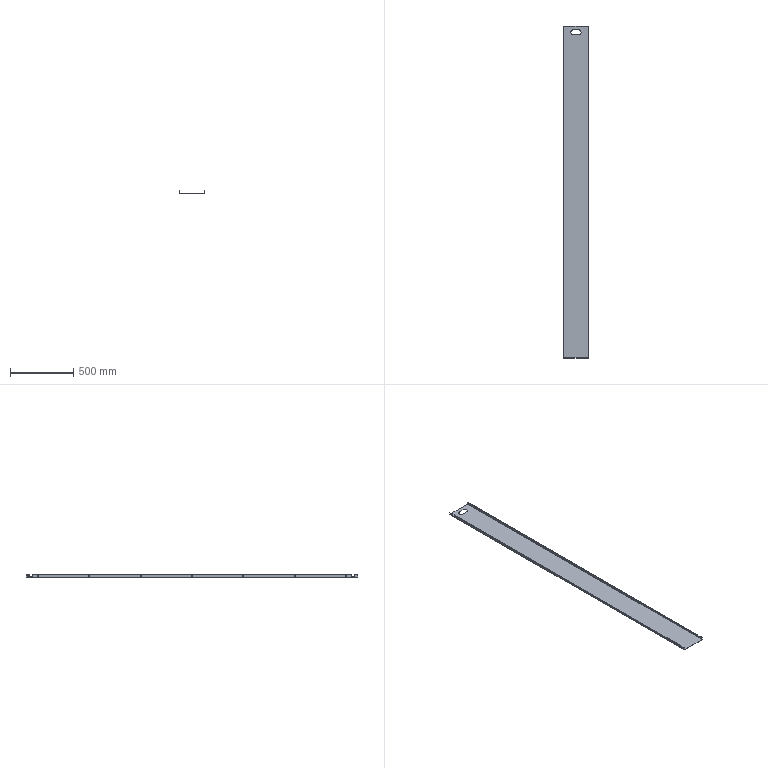Part | 1 solid | 93 faces | box 200 x 2616 x 20 mm | volume 920292 mm3 | plane 50 | cylinder 43 | commonest cylinder face diameters 6.2 x28 10 x8 40 x3 0.4 x2 3.4 x2